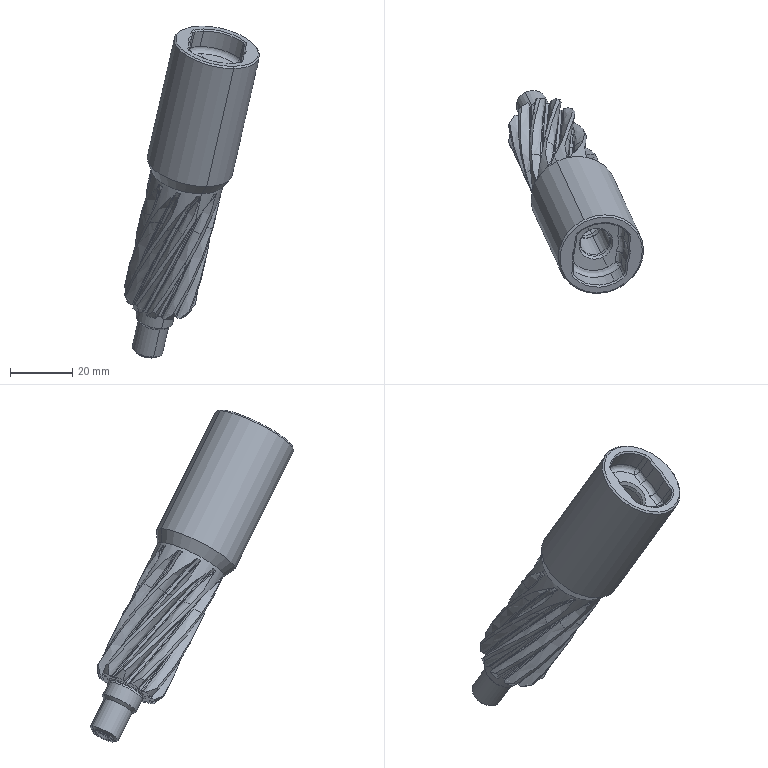Part | SolidWorks | features BaseBody 1 | 1 solid | 264 faces | box 43.345 x 65.256 x 106.487 mm | volume 42238 mm3 | spline 162 | cone 50 | cylinder 30 | plane 12 | torus 10 | commonest cylinder face diameters 4 x6 23.6 x6 22 x4 2.5 x2 9.5 x2 9.65 x2